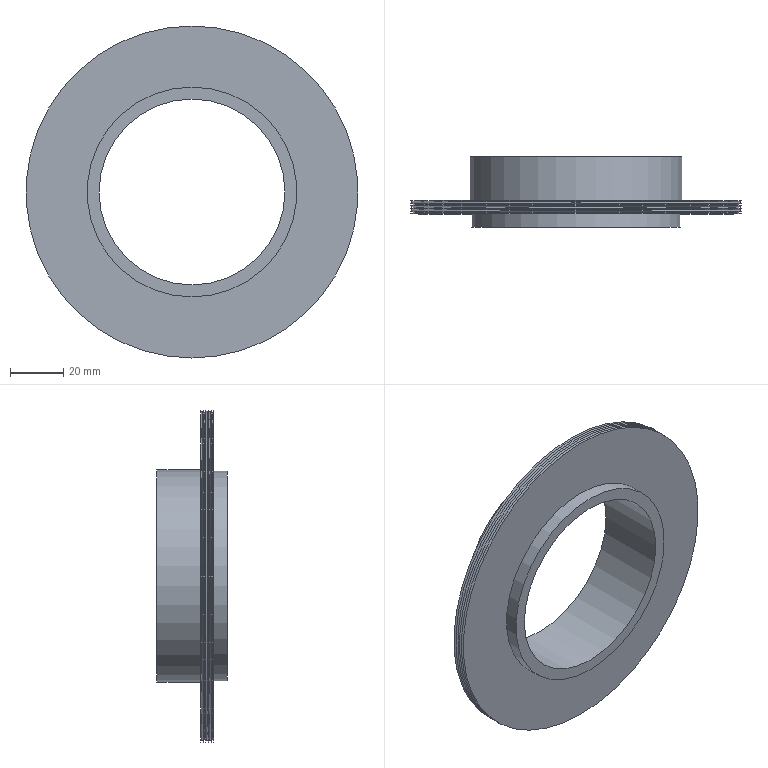Part | NX | 1 solid | 17 faces | box 125 x 26.5 x 125 mm | volume 65845 mm3 | cone 10 | plane 4 | cylinder 3 | commonest cylinder face diameters 70 x1 79 x1 80 x1
STEP:
#1=CARTESIAN_POINT('',(0.,39.,40.));
#2=VERTEX_POINT('',#1);
#3=CARTESIAN_POINT('',(0.,39.,0.));
#4=DIRECTION('',(0.,1.,0.));
#5=DIRECTION('',(0.,0.,1.));
#6=AXIS2_PLACEMENT_3D('',#3,#4,#5);
#7=CIRCLE('',#6,40.);
#8=EDGE_CURVE('',#2,#2,#7,.T.);
#9=ORIENTED_EDGE('',*,*,#8,.T.);
#10=EDGE_LOOP('',(#9));
#11=FACE_BOUND('',#10,.T.);
#12=CARTESIAN_POINT('',(0.,55.5,40.));
#13=VERTEX_POINT('',#12);
#14=CARTESIAN_POINT('',(0.,55.5,0.));
#15=DIRECTION('',(0.,1.,0.));
#16=DIRECTION('',(0.,0.,1.));
#17=AXIS2_PLACEMENT_3D('',#14,#15,#16);
#18=CIRCLE('',#17,40.);
#19=EDGE_CURVE('',#13,#13,#18,.T.);
#20=ORIENTED_EDGE('',*,*,#19,.F.);
#21=EDGE_LOOP('',(#20));
#22=FACE_BOUND('',#21,.T.);
#23=CARTESIAN_POINT('',(0.,0.,0.));
#24=DIRECTION('',(0.,1.,0.));
#25=DIRECTION('',(0.,0.,-1.));
#26=AXIS2_PLACEMENT_3D('',#23,#24,#25);
#27=CYLINDRICAL_SURFACE('',#26,40.);
#28=ADVANCED_FACE('',(#11,#22),#27,.T.);
#29=CARTESIAN_POINT('',(0.,39.,62.5));
#30=VERTEX_POINT('',#29);
#31=CARTESIAN_POINT('',(0.,39.,0.));
#32=DIRECTION('',(0.,1.,0.));
#33=DIRECTION('',(0.,0.,1.));
#34=AXIS2_PLACEMENT_3D('',#31,#32,#33);
#35=CIRCLE('',#34,62.5);
#36=EDGE_CURVE('',#30,#30,#35,.T.);
#37=ORIENTED_EDGE('',*,*,#36,.T.);
#38=EDGE_LOOP('',(#37));
#39=FACE_BOUND('',#38,.T.);
#40=ORIENTED_EDGE('',*,*,#8,.F.);
#41=EDGE_LOOP('',(#40));
#42=FACE_BOUND('',#41,.T.);
#43=CARTESIAN_POINT('',(40.,39.,0.));
#44=DIRECTION('',(0.,1.,0.));
#45=DIRECTION('',(0.,0.,-1.));
#46=AXIS2_PLACEMENT_3D('',#43,#44,#45);
#47=PLANE('',#46);
#48=ADVANCED_FACE('',(#39,#42),#47,.T.);
#49=CARTESIAN_POINT('',(0.,38.5,61.5));
#50=VERTEX_POINT('',#49);
#51=CARTESIAN_POINT('',(0.,38.5,0.));
#52=DIRECTION('',(0.,1.,0.));
#53=DIRECTION('',(0.,0.,1.));
#54=AXIS2_PLACEMENT_3D('',#51,#52,#53);
#55=CIRCLE('',#54,61.5);
#56=EDGE_CURVE('',#50,#50,#55,.T.);
#57=ORIENTED_EDGE('',*,*,#56,.T.);
#58=EDGE_LOOP('',(#57));
#59=FACE_BOUND('',#58,.T.);
#60=ORIENTED_EDGE('',*,*,#36,.F.);
#61=EDGE_LOOP('',(#60));
#62=FACE_BOUND('',#61,.T.);
#63=CARTESIAN_POINT('',(0.,39.,0.));
#64=DIRECTION('',(0.,1.,0.));
#65=DIRECTION('',(0.,0.,-1.));
#66=AXIS2_PLACEMENT_3D('',#63,#64,#65);
#67=CONICAL_SURFACE('',#66,62.5,63.435);
#68=ADVANCED_FACE('',(#59,#62),#67,.T.);
#69=CARTESIAN_POINT('',(0.,38.,62.5));
#70=VERTEX_POINT('',#69);
#71=CARTESIAN_POINT('',(0.,38.,0.));
#72=DIRECTION('',(0.,1.,0.));
#73=DIRECTION('',(0.,0.,1.));
#74=AXIS2_PLACEMENT_3D('',#71,#72,#73);
#75=CIRCLE('',#74,62.5);
#76=EDGE_CURVE('',#70,#70,#75,.T.);
#77=ORIENTED_EDGE('',*,*,#76,.T.);
#78=EDGE_LOOP('',(#77));
#79=FACE_BOUND('',#78,.T.);
#80=ORIENTED_EDGE('',*,*,#56,.F.);
#81=EDGE_LOOP('',(#80));
#82=FACE_BOUND('',#81,.T.);
#83=CARTESIAN_POINT('',(0.,38.5,0.));
#84=DIRECTION('',(0.,-1.,0.));
#85=DIRECTION('',(0.,0.,1.));
#86=AXIS2_PLACEMENT_3D('',#83,#84,#85);
#87=CONICAL_SURFACE('',#86,61.5,63.435);
#88=ADVANCED_FACE('',(#79,#82),#87,.T.);
#89=CARTESIAN_POINT('',(0.,37.5,61.5));
#90=VERTEX_POINT('',#89);
#91=CARTESIAN_POINT('',(0.,37.5,0.));
#92=DIRECTION('',(0.,1.,0.));
#93=DIRECTION('',(0.,0.,1.));
#94=AXIS2_PLACEMENT_3D('',#91,#92,#93);
#95=CIRCLE('',#94,61.5);
#96=EDGE_CURVE('',#90,#90,#95,.T.);
#97=ORIENTED_EDGE('',*,*,#96,.T.);
#98=EDGE_LOOP('',(#97));
#99=FACE_BOUND('',#98,.T.);
#100=ORIENTED_EDGE('',*,*,#76,.F.);
#101=EDGE_LOOP('',(#100));
#102=FACE_BOUND('',#101,.T.);
#103=CARTESIAN_POINT('',(0.,38.,0.));
#104=DIRECTION('',(0.,1.,0.));
#105=DIRECTION('',(0.,0.,-1.));
#106=AXIS2_PLACEMENT_3D('',#103,#104,#105);
#107=CONICAL_SURFACE('',#106,62.5,63.435);
#108=ADVANCED_FACE('',(#99,#102),#107,.T.);
#109=CARTESIAN_POINT('',(0.,37.,62.5));
#110=VERTEX_POINT('',#109);
#111=CARTESIAN_POINT('',(0.,37.,0.));
#112=DIRECTION('',(0.,1.,0.));
#113=DIRECTION('',(0.,0.,1.));
#114=AXIS2_PLACEMENT_3D('',#111,#112,#113);
#115=CIRCLE('',#114,62.5);
#116=EDGE_CURVE('',#110,#110,#115,.T.);
#117=ORIENTED_EDGE('',*,*,#116,.T.);
#118=EDGE_LOOP('',(#117));
#119=FACE_BOUND('',#118,.T.);
#120=ORIENTED_EDGE('',*,*,#96,.F.);
#121=EDGE_LOOP('',(#120));
#122=FACE_BOUND('',#121,.T.);
#123=CARTESIAN_POINT('',(0.,37.5,0.));
#124=DIRECTION('',(0.,-1.,0.));
#125=DIRECTION('',(0.,0.,1.));
#126=AXIS2_PLACEMENT_3D('',#123,#124,#125);
#127=CONICAL_SURFACE('',#126,61.5,63.435);
#128=ADVANCED_FACE('',(#119,#122),#127,.T.);
#129=CARTESIAN_POINT('',(0.,36.5,61.5));
#130=VERTEX_POINT('',#129);
#131=CARTESIAN_POINT('',(0.,36.5,0.));
#132=DIRECTION('',(0.,1.,0.));
#133=DIRECTION('',(0.,0.,1.));
#134=AXIS2_PLACEMENT_3D('',#131,#132,#133);
#135=CIRCLE('',#134,61.5);
#136=EDGE_CURVE('',#130,#130,#135,.T.);
#137=ORIENTED_EDGE('',*,*,#136,.T.);
#138=EDGE_LOOP('',(#137));
#139=FACE_BOUND('',#138,.T.);
#140=ORIENTED_EDGE('',*,*,#116,.F.);
#141=EDGE_LOOP('',(#140));
#142=FACE_BOUND('',#141,.T.);
#143=CARTESIAN_POINT('',(0.,37.,0.));
#144=DIRECTION('',(0.,1.,0.));
#145=DIRECTION('',(0.,0.,-1.));
#146=AXIS2_PLACEMENT_3D('',#143,#144,#145);
#147=CONICAL_SURFACE('',#146,62.5,63.435);
#148=ADVANCED_FACE('',(#139,#142),#147,.T.);
#149=CARTESIAN_POINT('',(0.,36.,62.5));
#150=VERTEX_POINT('',#149);
#151=CARTESIAN_POINT('',(0.,36.,0.));
#152=DIRECTION('',(0.,1.,0.));
#153=DIRECTION('',(0.,0.,1.));
#154=AXIS2_PLACEMENT_3D('',#151,#152,#153);
#155=CIRCLE('',#154,62.5);
#156=EDGE_CURVE('',#150,#150,#155,.T.);
#157=ORIENTED_EDGE('',*,*,#156,.T.);
#158=EDGE_LOOP('',(#157));
#159=FACE_BOUND('',#158,.T.);
#160=ORIENTED_EDGE('',*,*,#136,.F.);
#161=EDGE_LOOP('',(#160));
#162=FACE_BOUND('',#161,.T.);
#163=CARTESIAN_POINT('',(0.,36.5,0.));
#164=DIRECTION('',(0.,-1.,0.));
#165=DIRECTION('',(0.,0.,1.));
#166=AXIS2_PLACEMENT_3D('',#163,#164,#165);
#167=CONICAL_SURFACE('',#166,61.5,63.435);
#168=ADVANCED_FACE('',(#159,#162),#167,.T.);
#169=CARTESIAN_POINT('',(0.,35.5,61.5));
#170=VERTEX_POINT('',#169);
#171=CARTESIAN_POINT('',(0.,35.5,0.));
#172=DIRECTION('',(0.,1.,0.));
#173=DIRECTION('',(0.,0.,1.));
#174=AXIS2_PLACEMENT_3D('',#171,#172,#173);
#175=CIRCLE('',#174,61.5);
#176=EDGE_CURVE('',#170,#170,#175,.T.);
#177=ORIENTED_EDGE('',*,*,#176,.T.);
#178=EDGE_LOOP('',(#177));
#179=FACE_BOUND('',#178,.T.);
#180=ORIENTED_EDGE('',*,*,#156,.F.);
#181=EDGE_LOOP('',(#180));
#182=FACE_BOUND('',#181,.T.);
#183=CARTESIAN_POINT('',(0.,36.,0.));
#184=DIRECTION('',(0.,1.,0.));
#185=DIRECTION('',(0.,0.,-1.));
#186=AXIS2_PLACEMENT_3D('',#183,#184,#185);
#187=CONICAL_SURFACE('',#186,62.5,63.435);
#188=ADVANCED_FACE('',(#179,#182),#187,.T.);
#189=CARTESIAN_POINT('',(0.,35.,62.5));
#190=VERTEX_POINT('',#189);
#191=CARTESIAN_POINT('',(0.,35.,0.));
#192=DIRECTION('',(0.,1.,0.));
#193=DIRECTION('',(0.,0.,1.));
#194=AXIS2_PLACEMENT_3D('',#191,#192,#193);
#195=CIRCLE('',#194,62.5);
#196=EDGE_CURVE('',#190,#190,#195,.T.);
#197=ORIENTED_EDGE('',*,*,#196,.T.);
#198=EDGE_LOOP('',(#197));
#199=FACE_BOUND('',#198,.T.);
#200=ORIENTED_EDGE('',*,*,#176,.F.);
#201=EDGE_LOOP('',(#200));
#202=FACE_BOUND('',#201,.T.);
#203=CARTESIAN_POINT('',(0.,35.5,0.));
#204=DIRECTION('',(0.,-1.,0.));
#205=DIRECTION('',(0.,0.,1.));
#206=AXIS2_PLACEMENT_3D('',#203,#204,#205);
#207=CONICAL_SURFACE('',#206,61.5,63.435);
#208=ADVANCED_FACE('',(#199,#202),#207,.T.);
#209=CARTESIAN_POINT('',(0.,34.5,61.5));
#210=VERTEX_POINT('',#209);
#211=CARTESIAN_POINT('',(0.,34.5,0.));
#212=DIRECTION('',(0.,1.,0.));
#213=DIRECTION('',(0.,0.,1.));
#214=AXIS2_PLACEMENT_3D('',#211,#212,#213);
#215=CIRCLE('',#214,61.5);
#216=EDGE_CURVE('',#210,#210,#215,.T.);
#217=ORIENTED_EDGE('',*,*,#216,.T.);
#218=EDGE_LOOP('',(#217));
#219=FACE_BOUND('',#218,.T.);
#220=ORIENTED_EDGE('',*,*,#196,.F.);
#221=EDGE_LOOP('',(#220));
#222=FACE_BOUND('',#221,.T.);
#223=CARTESIAN_POINT('',(0.,35.,0.));
#224=DIRECTION('',(0.,1.,0.));
#225=DIRECTION('',(0.,0.,-1.));
#226=AXIS2_PLACEMENT_3D('',#223,#224,#225);
#227=CONICAL_SURFACE('',#226,62.5,63.435);
#228=ADVANCED_FACE('',(#219,#222),#227,.T.);
#229=CARTESIAN_POINT('',(0.,34.,62.5));
#230=VERTEX_POINT('',#229);
#231=CARTESIAN_POINT('',(0.,34.,0.));
#232=DIRECTION('',(0.,1.,0.));
#233=DIRECTION('',(0.,0.,1.));
#234=AXIS2_PLACEMENT_3D('',#231,#232,#233);
#235=CIRCLE('',#234,62.5);
#236=EDGE_CURVE('',#230,#230,#235,.T.);
#237=ORIENTED_EDGE('',*,*,#236,.T.);
#238=EDGE_LOOP('',(#237));
#239=FACE_BOUND('',#238,.T.);
#240=ORIENTED_EDGE('',*,*,#216,.F.);
#241=EDGE_LOOP('',(#240));
#242=FACE_BOUND('',#241,.T.);
#243=CARTESIAN_POINT('',(0.,34.5,0.));
#244=DIRECTION('',(0.,-1.,0.));
#245=DIRECTION('',(0.,0.,1.));
#246=AXIS2_PLACEMENT_3D('',#243,#244,#245);
#247=CONICAL_SURFACE('',#246,61.5,63.435);
#248=ADVANCED_FACE('',(#239,#242),#247,.T.);
#249=CARTESIAN_POINT('',(0.,34.,39.5));
#250=VERTEX_POINT('',#249);
#251=CARTESIAN_POINT('',(0.,34.,0.));
#252=DIRECTION('',(0.,1.,0.));
#253=DIRECTION('',(0.,0.,1.));
#254=AXIS2_PLACEMENT_3D('',#251,#252,#253);
#255=CIRCLE('',#254,39.5);
#256=EDGE_CURVE('',#250,#250,#255,.T.);
#257=ORIENTED_EDGE('',*,*,#256,.T.);
#258=EDGE_LOOP('',(#257));
#259=FACE_BOUND('',#258,.T.);
#260=ORIENTED_EDGE('',*,*,#236,.F.);
#261=EDGE_LOOP('',(#260));
#262=FACE_BOUND('',#261,.T.);
#263=CARTESIAN_POINT('',(62.5,34.,0.));
#264=DIRECTION('',(0.,-1.,0.));
#265=DIRECTION('',(0.,0.,1.));
#266=AXIS2_PLACEMENT_3D('',#263,#264,#265);
#267=PLANE('',#266);
#268=ADVANCED_FACE('',(#259,#262),#267,.T.);
#269=CARTESIAN_POINT('',(0.,29.,39.5));
#270=VERTEX_POINT('',#269);
#271=CARTESIAN_POINT('',(0.,29.,0.));
#272=DIRECTION('',(0.,1.,0.));
#273=DIRECTION('',(0.,0.,1.));
#274=AXIS2_PLACEMENT_3D('',#271,#272,#273);
#275=CIRCLE('',#274,39.5);
#276=EDGE_CURVE('',#270,#270,#275,.T.);
#277=ORIENTED_EDGE('',*,*,#276,.T.);
#278=EDGE_LOOP('',(#277));
#279=FACE_BOUND('',#278,.T.);
#280=ORIENTED_EDGE('',*,*,#256,.F.);
#281=EDGE_LOOP('',(#280));
#282=FACE_BOUND('',#281,.T.);
#283=CARTESIAN_POINT('',(0.,0.,0.));
#284=DIRECTION('',(0.,1.,0.));
#285=DIRECTION('',(0.,0.,-1.));
#286=AXIS2_PLACEMENT_3D('',#283,#284,#285);
#287=CYLINDRICAL_SURFACE('',#286,39.5);
#288=ADVANCED_FACE('',(#279,#282),#287,.T.);
#289=CARTESIAN_POINT('',(0.,29.,35.));
#290=VERTEX_POINT('',#289);
#291=CARTESIAN_POINT('',(0.,29.,0.));
#292=DIRECTION('',(0.,1.,0.));
#293=DIRECTION('',(0.,0.,1.));
#294=AXIS2_PLACEMENT_3D('',#291,#292,#293);
#295=CIRCLE('',#294,35.);
#296=EDGE_CURVE('',#290,#290,#295,.T.);
#297=ORIENTED_EDGE('',*,*,#296,.T.);
#298=EDGE_LOOP('',(#297));
#299=FACE_BOUND('',#298,.T.);
#300=ORIENTED_EDGE('',*,*,#276,.F.);
#301=EDGE_LOOP('',(#300));
#302=FACE_BOUND('',#301,.T.);
#303=CARTESIAN_POINT('',(39.5,29.,0.));
#304=DIRECTION('',(0.,-1.,0.));
#305=DIRECTION('',(0.,0.,1.));
#306=AXIS2_PLACEMENT_3D('',#303,#304,#305);
#307=PLANE('',#306);
#308=ADVANCED_FACE('',(#299,#302),#307,.T.);
#309=CARTESIAN_POINT('',(0.,55.5,35.));
#310=VERTEX_POINT('',#309);
#311=CARTESIAN_POINT('',(0.,55.5,0.));
#312=DIRECTION('',(0.,1.,0.));
#313=DIRECTION('',(0.,0.,1.));
#314=AXIS2_PLACEMENT_3D('',#311,#312,#313);
#315=CIRCLE('',#314,35.);
#316=EDGE_CURVE('',#310,#310,#315,.T.);
#317=ORIENTED_EDGE('',*,*,#316,.T.);
#318=EDGE_LOOP('',(#317));
#319=FACE_BOUND('',#318,.T.);
#320=ORIENTED_EDGE('',*,*,#296,.F.);
#321=EDGE_LOOP('',(#320));
#322=FACE_BOUND('',#321,.T.);
#323=CARTESIAN_POINT('',(0.,0.,0.));
#324=DIRECTION('',(0.,1.,0.));
#325=DIRECTION('',(0.,0.,-1.));
#326=AXIS2_PLACEMENT_3D('',#323,#324,#325);
#327=CYLINDRICAL_SURFACE('',#326,35.);
#328=ADVANCED_FACE('',(#319,#322),#327,.F.);
#329=ORIENTED_EDGE('',*,*,#19,.T.);
#330=EDGE_LOOP('',(#329));
#331=FACE_BOUND('',#330,.T.);
#332=ORIENTED_EDGE('',*,*,#316,.F.);
#333=EDGE_LOOP('',(#332));
#334=FACE_BOUND('',#333,.T.);
#335=CARTESIAN_POINT('',(35.,55.5,0.));
#336=DIRECTION('',(0.,1.,0.));
#337=DIRECTION('',(0.,0.,-1.));
#338=AXIS2_PLACEMENT_3D('',#335,#336,#337);
#339=PLANE('',#338);
#340=ADVANCED_FACE('',(#331,#334),#339,.T.);
#341=CLOSED_SHELL('',(#28,#48,#68,#88,#108,#128,#148,#168,#188,#208,#228,#248,#268,#288,#308,#328,#340));
#342=MANIFOLD_SOLID_BREP('',#341);
#343=(LENGTH_UNIT()NAMED_UNIT(*)SI_UNIT(.MILLI.,.METRE.));
#344=UNCERTAINTY_MEASURE_WITH_UNIT(LENGTH_MEASURE(0.00002),#343,'','');
#345=(NAMED_UNIT(*)PLANE_ANGLE_UNIT()SI_UNIT($,.RADIAN.));
#346=PLANE_ANGLE_MEASURE_WITH_UNIT(PLANE_ANGLE_MEASURE(0.01745),#345);
#347=DIMENSIONAL_EXPONENTS(0.,0.,0.,0.,0.,0.,0.);
#348=(CONVERSION_BASED_UNIT('DEGREE',#346)NAMED_UNIT(#347)PLANE_ANGLE_UNIT());
#349=(NAMED_UNIT(*)SI_UNIT($,.STERADIAN.)SOLID_ANGLE_UNIT());
#350=(GEOMETRIC_REPRESENTATION_CONTEXT(3)GLOBAL_UNCERTAINTY_ASSIGNED_CONTEXT((#344))GLOBAL_UNIT_ASSIGNED_CONTEXT((#343,#348,#349))REPRESENTATION_CONTEXT('',''));
#351=ADVANCED_BREP_SHAPE_REPRESENTATION('',(#342),#350);